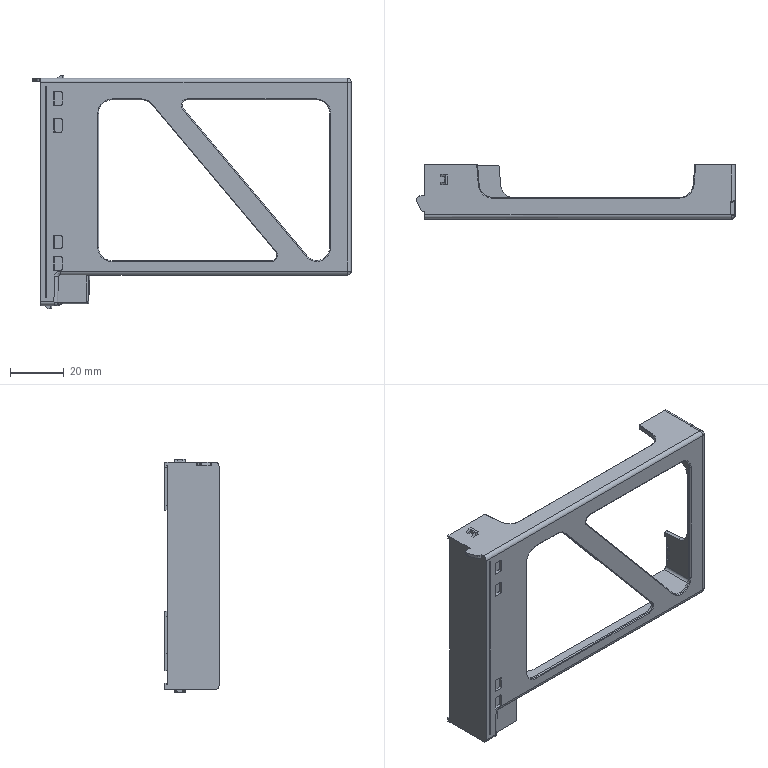Part | SolidWorks | features BaseBody 1 | 1 solid | 296 faces | box 118.5 x 20.1 x 87 mm | volume 34968 mm3 | plane 167 | cylinder 92 | spline 35 | torus 2 | commonest cylinder face diameters 0.6 x33 0.8 x16 3 x14 10 x12 2 x10 1 x5